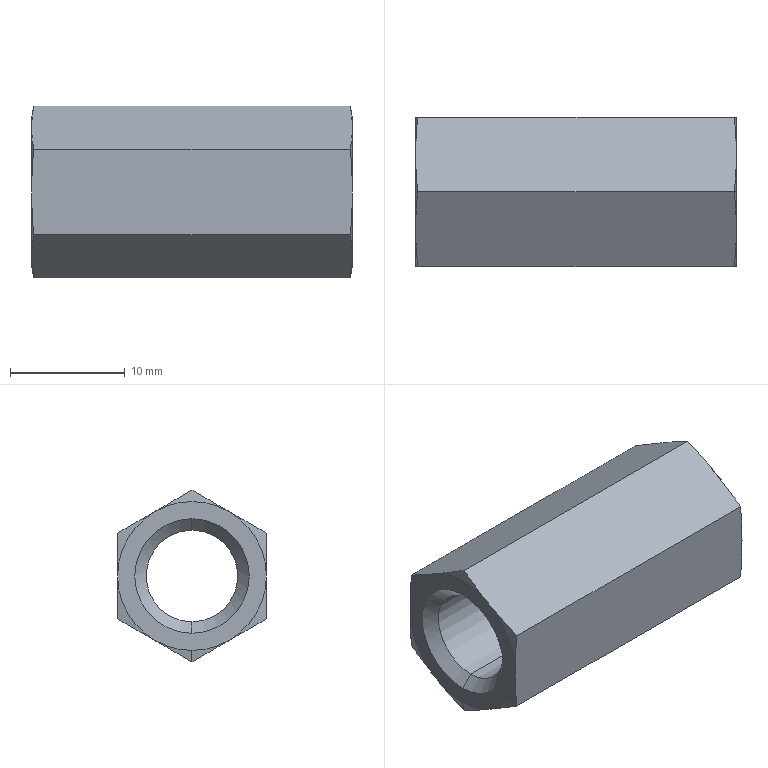Part | STEP file | 1 solid | 28 faces | box 28 x 13 x 15.011 mm | volume 2662 mm3 | cone 18 | plane 8 | cylinder 2 | commonest cylinder face diameters 8 x2